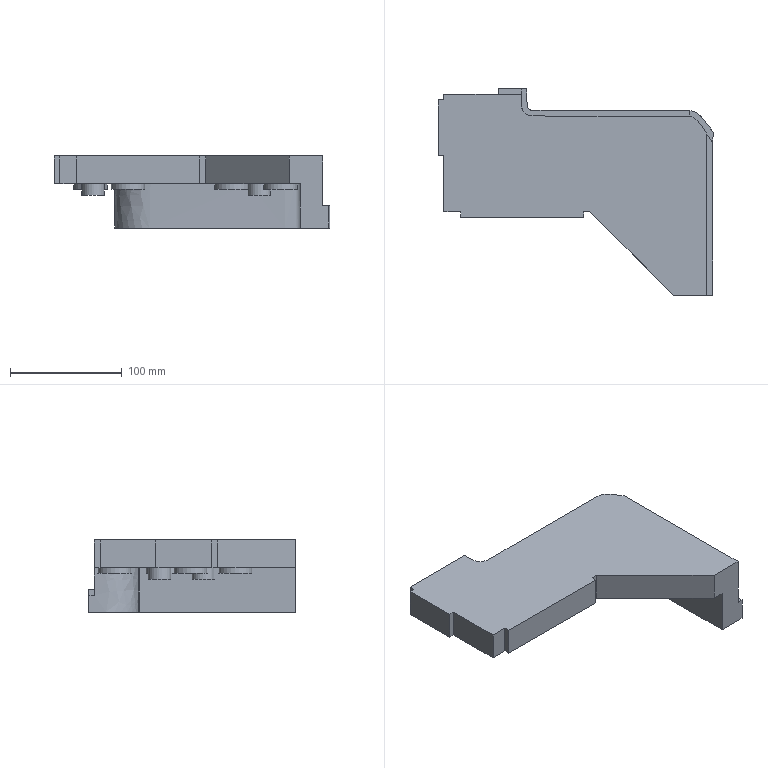Part | NX | features solid 2 | 1 solid | 44 faces | box 246.215 x 184.392 x 64.5 mm | volume 1009232 mm3 | plane 26 | spline 12 | cylinder 6 | commonest cylinder face diameters 30 x4 20 x2